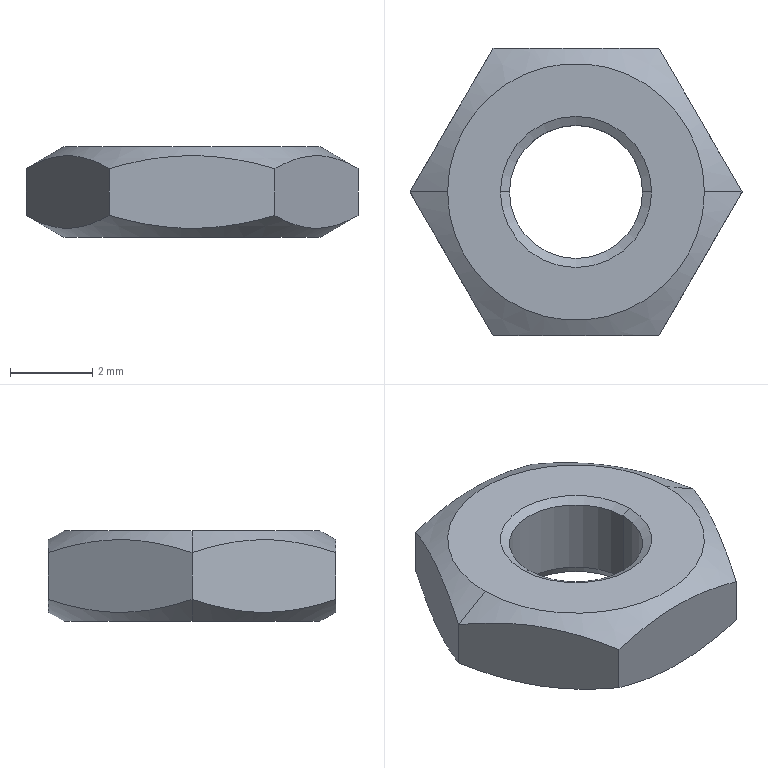Part | SolidWorks | features RevCut 2, Chamfer 1, Extrusion 1, LPattern 1 | 1 solid | 18 faces | box 8.083 x 7 x 2.2 mm | volume 70.72 mm3 | cone 8 | plane 8 | cylinder 2 | commonest cylinder face diameters 3.242 x2
STEP:
#1=CARTESIAN_POINT('',(-1.621,0.,-0.127));
#2=VERTEX_POINT('',#1);
#3=CARTESIAN_POINT('',(1.621,0.,-0.127));
#4=VERTEX_POINT('',#3);
#5=CARTESIAN_POINT('',(0.,0.,-0.127));
#6=DIRECTION('',(0.,0.,1.));
#7=DIRECTION('',(1.,0.,0.));
#8=AXIS2_PLACEMENT_3D('',#5,#6,#7);
#9=CIRCLE('',#8,1.621);
#10=EDGE_CURVE('',#2,#4,#9,.T.);
#11=ORIENTED_EDGE('',*,*,#10,.F.);
#12=CARTESIAN_POINT('',(-1.841,0.,0.));
#13=VERTEX_POINT('',#12);
#14=CARTESIAN_POINT('',(-1.621,0.,-0.127));
#15=DIRECTION('',(-0.866,0.,0.5));
#16=VECTOR('',#15,1000.);
#17=LINE('',#14,#16);
#18=EDGE_CURVE('',#2,#13,#17,.T.);
#19=ORIENTED_EDGE('',*,*,#18,.T.);
#20=CARTESIAN_POINT('',(1.841,0.,0.));
#21=VERTEX_POINT('',#20);
#22=CARTESIAN_POINT('',(0.,0.,0.));
#23=DIRECTION('',(0.,0.,-1.));
#24=DIRECTION('',(1.,0.,0.));
#25=AXIS2_PLACEMENT_3D('',#22,#23,#24);
#26=CIRCLE('',#25,1.841);
#27=EDGE_CURVE('',#21,#13,#26,.T.);
#28=ORIENTED_EDGE('',*,*,#27,.F.);
#29=CARTESIAN_POINT('',(1.621,0.,-0.127));
#30=DIRECTION('',(0.866,0.,0.5));
#31=VECTOR('',#30,1000.);
#32=LINE('',#29,#31);
#33=EDGE_CURVE('',#4,#21,#32,.T.);
#34=ORIENTED_EDGE('',*,*,#33,.F.);
#35=EDGE_LOOP('',(#11,#19,#28,#34));
#36=FACE_OUTER_BOUND('',#35,.T.);
#37=CARTESIAN_POINT('',(0.,0.,-0.127));
#38=DIRECTION('',(0.,0.,1.));
#39=DIRECTION('',(1.,0.,0.));
#40=AXIS2_PLACEMENT_3D('',#37,#38,#39);
#41=CONICAL_SURFACE('',#40,1.621,1.047);
#42=ADVANCED_FACE('',(#36),#41,.F.);
#43=CARTESIAN_POINT('',(1.621,0.,-1.98));
#44=VERTEX_POINT('',#43);
#45=CARTESIAN_POINT('',(-1.621,0.,-1.98));
#46=VERTEX_POINT('',#45);
#47=CARTESIAN_POINT('',(0.,0.,-1.98));
#48=DIRECTION('',(0.,0.,-1.));
#49=DIRECTION('',(1.,0.,0.));
#50=AXIS2_PLACEMENT_3D('',#47,#48,#49);
#51=CIRCLE('',#50,1.621);
#52=EDGE_CURVE('',#44,#46,#51,.T.);
#53=ORIENTED_EDGE('',*,*,#52,.F.);
#54=CARTESIAN_POINT('',(1.748,0.,-2.2));
#55=VERTEX_POINT('',#54);
#56=CARTESIAN_POINT('',(1.748,0.,-2.2));
#57=DIRECTION('',(0.5,0.,-0.866));
#58=VECTOR('',#57,1000.);
#59=LINE('',#56,#58);
#60=EDGE_CURVE('',#44,#55,#59,.T.);
#61=ORIENTED_EDGE('',*,*,#60,.T.);
#62=CARTESIAN_POINT('',(-1.748,0.,-2.2));
#63=VERTEX_POINT('',#62);
#64=CARTESIAN_POINT('',(0.,0.,-2.2));
#65=DIRECTION('',(0.,0.,1.));
#66=DIRECTION('',(1.,0.,0.));
#67=AXIS2_PLACEMENT_3D('',#64,#65,#66);
#68=CIRCLE('',#67,1.748);
#69=EDGE_CURVE('',#63,#55,#68,.T.);
#70=ORIENTED_EDGE('',*,*,#69,.F.);
#71=CARTESIAN_POINT('',(-1.748,0.,-2.2));
#72=DIRECTION('',(-0.5,0.,-0.866));
#73=VECTOR('',#72,1000.);
#74=LINE('',#71,#73);
#75=EDGE_CURVE('',#46,#63,#74,.T.);
#76=ORIENTED_EDGE('',*,*,#75,.F.);
#77=EDGE_LOOP('',(#53,#61,#70,#76));
#78=FACE_OUTER_BOUND('',#77,.T.);
#79=CARTESIAN_POINT('',(0.,0.,-2.2));
#80=DIRECTION('',(0.,0.,-1.));
#81=DIRECTION('',(-1.,0.,0.));
#82=AXIS2_PLACEMENT_3D('',#79,#80,#81);
#83=CONICAL_SURFACE('',#82,1.748,0.5236);
#84=ADVANCED_FACE('',(#78),#83,.F.);
#85=CARTESIAN_POINT('',(-3.125,0.,0.));
#86=VERTEX_POINT('',#85);
#87=CARTESIAN_POINT('',(3.125,0.,0.));
#88=VERTEX_POINT('',#87);
#89=CARTESIAN_POINT('',(0.,0.,0.));
#90=DIRECTION('',(0.,0.,-1.));
#91=DIRECTION('',(-1.,0.,0.));
#92=AXIS2_PLACEMENT_3D('',#89,#90,#91);
#93=CIRCLE('',#92,3.125);
#94=EDGE_CURVE('',#86,#88,#93,.T.);
#95=ORIENTED_EDGE('',*,*,#94,.T.);
#96=CARTESIAN_POINT('',(4.041,0.,-0.5291));
#97=VERTEX_POINT('',#96);
#98=CARTESIAN_POINT('',(3.125,0.,0.));
#99=DIRECTION('',(0.866,0.,-0.5));
#100=VECTOR('',#99,1000.);
#101=LINE('',#98,#100);
#102=EDGE_CURVE('',#88,#97,#101,.T.);
#103=ORIENTED_EDGE('',*,*,#102,.T.);
#104=CARTESIAN_POINT('',(2.021,3.5,-0.5291));
#105=VERTEX_POINT('',#104);
#106=CARTESIAN_POINT('',(4.041,0.,-0.5291));
#107=CARTESIAN_POINT('',(3.712,0.5715,-0.3386));
#108=CARTESIAN_POINT('',(3.377,1.152,-0.2169));
#109=CARTESIAN_POINT('',(2.861,2.044,-0.2163));
#110=CARTESIAN_POINT('',(2.69,2.341,-0.2461));
#111=CARTESIAN_POINT('',(2.352,2.925,-0.3551));
#112=CARTESIAN_POINT('',(2.186,3.214,-0.4337));
#113=CARTESIAN_POINT('',(2.021,3.5,-0.5291));
#114=B_SPLINE_CURVE_WITH_KNOTS('',3,(#106,#107,#108,#109,#110,#111,#112,#113),.UNSPECIFIED.,.F.,.F.,(4,2,2,4),(0.000000238,0.002041,0.003061,0.004082),.UNSPECIFIED.);
#115=EDGE_CURVE('',#97,#105,#114,.T.);
#116=ORIENTED_EDGE('',*,*,#115,.T.);
#117=CARTESIAN_POINT('',(-2.021,3.5,-0.5291));
#118=VERTEX_POINT('',#117);
#119=CARTESIAN_POINT('',(2.021,3.5,-0.5291));
#120=CARTESIAN_POINT('',(1.694,3.5,-0.4348));
#121=CARTESIAN_POINT('',(1.363,3.5,-0.3563));
#122=CARTESIAN_POINT('',(0.6882,3.5,-0.2467));
#123=CARTESIAN_POINT('',(0.342,3.5,-0.2165));
#124=CARTESIAN_POINT('',(-0.3409,3.5,-0.2165));
#125=CARTESIAN_POINT('',(-0.6803,3.5,-0.2458));
#126=CARTESIAN_POINT('',(-1.355,3.5,-0.3546));
#127=CARTESIAN_POINT('',(-1.692,3.5,-0.4342));
#128=CARTESIAN_POINT('',(-2.021,3.5,-0.5291));
#129=B_SPLINE_CURVE_WITH_KNOTS('',3,(#119,#120,#121,#122,#123,#124,#125,#126,#127,#128),.UNSPECIFIED.,.F.,.F.,(4,2,2,2,4),(0.008992,0.01002,0.01104,0.01206,0.01309),.UNSPECIFIED.);
#130=EDGE_CURVE('',#105,#118,#129,.T.);
#131=ORIENTED_EDGE('',*,*,#130,.T.);
#132=CARTESIAN_POINT('',(-4.041,0.,-0.5291));
#133=VERTEX_POINT('',#132);
#134=CARTESIAN_POINT('',(-2.021,3.5,-0.5291));
#135=CARTESIAN_POINT('',(-2.351,2.929,-0.3386));
#136=CARTESIAN_POINT('',(-2.686,2.348,-0.2169));
#137=CARTESIAN_POINT('',(-3.201,1.456,-0.2163));
#138=CARTESIAN_POINT('',(-3.373,1.159,-0.2461));
#139=CARTESIAN_POINT('',(-3.71,0.5746,-0.3551));
#140=CARTESIAN_POINT('',(-3.876,0.2861,-0.4337));
#141=CARTESIAN_POINT('',(-4.041,0.,-0.5291));
#142=B_SPLINE_CURVE_WITH_KNOTS('',3,(#134,#135,#136,#137,#138,#139,#140,#141),.UNSPECIFIED.,.F.,.F.,(4,2,2,4),(0.000000238,0.002041,0.003061,0.004082),.UNSPECIFIED.);
#143=EDGE_CURVE('',#118,#133,#142,.T.);
#144=ORIENTED_EDGE('',*,*,#143,.T.);
#145=CARTESIAN_POINT('',(-3.125,0.,0.));
#146=DIRECTION('',(-0.866,0.,-0.5));
#147=VECTOR('',#146,1000.);
#148=LINE('',#145,#147);
#149=EDGE_CURVE('',#86,#133,#148,.T.);
#150=ORIENTED_EDGE('',*,*,#149,.F.);
#151=EDGE_LOOP('',(#95,#103,#116,#131,#144,#150));
#152=FACE_OUTER_BOUND('',#151,.T.);
#153=CARTESIAN_POINT('',(0.,0.,0.));
#154=DIRECTION('',(0.,0.,-1.));
#155=DIRECTION('',(-1.,0.,0.));
#156=AXIS2_PLACEMENT_3D('',#153,#154,#155);
#157=CONICAL_SURFACE('',#156,3.125,1.047);
#158=ADVANCED_FACE('',(#152),#157,.T.);
#159=CARTESIAN_POINT('',(-3.125,0.,-2.2));
#160=VERTEX_POINT('',#159);
#161=CARTESIAN_POINT('',(3.125,0.,-2.2));
#162=VERTEX_POINT('',#161);
#163=CARTESIAN_POINT('',(0.,0.,-2.2));
#164=DIRECTION('',(0.,0.,-1.));
#165=DIRECTION('',(-1.,0.,0.));
#166=AXIS2_PLACEMENT_3D('',#163,#164,#165);
#167=CIRCLE('',#166,3.125);
#168=EDGE_CURVE('',#160,#162,#167,.T.);
#169=ORIENTED_EDGE('',*,*,#168,.F.);
#170=CARTESIAN_POINT('',(-4.041,0.,-1.671));
#171=VERTEX_POINT('',#170);
#172=CARTESIAN_POINT('',(-4.041,0.,-1.671));
#173=DIRECTION('',(-0.866,0.,0.5));
#174=VECTOR('',#173,1000.);
#175=LINE('',#172,#174);
#176=EDGE_CURVE('',#160,#171,#175,.T.);
#177=ORIENTED_EDGE('',*,*,#176,.T.);
#178=CARTESIAN_POINT('',(-2.021,3.5,-1.671));
#179=VERTEX_POINT('',#178);
#180=CARTESIAN_POINT('',(-4.041,0.,-1.671));
#181=CARTESIAN_POINT('',(-3.712,0.5715,-1.861));
#182=CARTESIAN_POINT('',(-3.377,1.152,-1.983));
#183=CARTESIAN_POINT('',(-2.861,2.044,-1.984));
#184=CARTESIAN_POINT('',(-2.69,2.341,-1.954));
#185=CARTESIAN_POINT('',(-2.352,2.925,-1.845));
#186=CARTESIAN_POINT('',(-2.186,3.214,-1.766));
#187=CARTESIAN_POINT('',(-2.021,3.5,-1.671));
#188=B_SPLINE_CURVE_WITH_KNOTS('',3,(#180,#181,#182,#183,#184,#185,#186,#187),.UNSPECIFIED.,.F.,.F.,(4,2,2,4),(0.000000238,0.002041,0.003061,0.004082),.UNSPECIFIED.);
#189=EDGE_CURVE('',#171,#179,#188,.T.);
#190=ORIENTED_EDGE('',*,*,#189,.T.);
#191=CARTESIAN_POINT('',(2.021,3.5,-1.671));
#192=VERTEX_POINT('',#191);
#193=CARTESIAN_POINT('',(-2.021,3.5,-1.671));
#194=CARTESIAN_POINT('',(-1.692,3.5,-1.766));
#195=CARTESIAN_POINT('',(-1.355,3.5,-1.845));
#196=CARTESIAN_POINT('',(-0.6803,3.5,-1.954));
#197=CARTESIAN_POINT('',(-0.3409,3.5,-1.984));
#198=CARTESIAN_POINT('',(0.342,3.5,-1.983));
#199=CARTESIAN_POINT('',(0.6882,3.5,-1.953));
#200=CARTESIAN_POINT('',(1.363,3.5,-1.844));
#201=CARTESIAN_POINT('',(1.694,3.5,-1.765));
#202=CARTESIAN_POINT('',(2.021,3.5,-1.671));
#203=B_SPLINE_CURVE_WITH_KNOTS('',3,(#193,#194,#195,#196,#197,#198,#199,#200,#201,#202),.UNSPECIFIED.,.F.,.F.,(4,2,2,2,4),(0.003572,0.004594,0.005616,0.006639,0.007661),.UNSPECIFIED.);
#204=EDGE_CURVE('',#179,#192,#203,.T.);
#205=ORIENTED_EDGE('',*,*,#204,.T.);
#206=CARTESIAN_POINT('',(4.041,0.,-1.671));
#207=VERTEX_POINT('',#206);
#208=CARTESIAN_POINT('',(2.021,3.5,-1.671));
#209=CARTESIAN_POINT('',(2.351,2.929,-1.861));
#210=CARTESIAN_POINT('',(2.686,2.348,-1.983));
#211=CARTESIAN_POINT('',(3.201,1.456,-1.984));
#212=CARTESIAN_POINT('',(3.373,1.159,-1.954));
#213=CARTESIAN_POINT('',(3.71,0.5746,-1.845));
#214=CARTESIAN_POINT('',(3.876,0.2861,-1.766));
#215=CARTESIAN_POINT('',(4.041,0.,-1.671));
#216=B_SPLINE_CURVE_WITH_KNOTS('',3,(#208,#209,#210,#211,#212,#213,#214,#215),.UNSPECIFIED.,.F.,.F.,(4,2,2,4),(0.000000238,0.002041,0.003061,0.004082),.UNSPECIFIED.);
#217=EDGE_CURVE('',#192,#207,#216,.T.);
#218=ORIENTED_EDGE('',*,*,#217,.T.);
#219=CARTESIAN_POINT('',(4.041,0.,-1.671));
#220=DIRECTION('',(0.866,0.,0.5));
#221=VECTOR('',#220,1000.);
#222=LINE('',#219,#221);
#223=EDGE_CURVE('',#162,#207,#222,.T.);
#224=ORIENTED_EDGE('',*,*,#223,.F.);
#225=EDGE_LOOP('',(#169,#177,#190,#205,#218,#224));
#226=FACE_OUTER_BOUND('',#225,.T.);
#227=CARTESIAN_POINT('',(0.,0.,-1.671));
#228=DIRECTION('',(0.,0.,1.));
#229=DIRECTION('',(1.,0.,0.));
#230=AXIS2_PLACEMENT_3D('',#227,#228,#229);
#231=CONICAL_SURFACE('',#230,4.041,1.047);
#232=ADVANCED_FACE('',(#226),#231,.T.);
#233=ORIENTED_EDGE('',*,*,#52,.T.);
#234=CARTESIAN_POINT('',(-1.621,0.,-2.2));
#235=DIRECTION('',(0.,0.,1.));
#236=VECTOR('',#235,1000.);
#237=LINE('',#234,#236);
#238=EDGE_CURVE('',#46,#2,#237,.T.);
#239=ORIENTED_EDGE('',*,*,#238,.T.);
#240=ORIENTED_EDGE('',*,*,#10,.T.);
#241=CARTESIAN_POINT('',(1.621,0.,-2.2));
#242=DIRECTION('',(0.,0.,1.));
#243=VECTOR('',#242,1000.);
#244=LINE('',#241,#243);
#245=EDGE_CURVE('',#44,#4,#244,.T.);
#246=ORIENTED_EDGE('',*,*,#245,.F.);
#247=EDGE_LOOP('',(#233,#239,#240,#246));
#248=FACE_OUTER_BOUND('',#247,.T.);
#249=CARTESIAN_POINT('',(0.,0.,-2.2));
#250=DIRECTION('',(0.,0.,1.));
#251=DIRECTION('',(1.,0.,0.));
#252=AXIS2_PLACEMENT_3D('',#249,#250,#251);
#253=CYLINDRICAL_SURFACE('',#252,1.621);
#254=ADVANCED_FACE('',(#248),#253,.F.);
#255=CARTESIAN_POINT('',(-2.021,-3.5,-0.5291));
#256=VERTEX_POINT('',#255);
#257=CARTESIAN_POINT('',(2.021,-3.5,-0.5291));
#258=VERTEX_POINT('',#257);
#259=CARTESIAN_POINT('',(-2.021,-3.5,-0.5291));
#260=CARTESIAN_POINT('',(-1.692,-3.5,-0.4342));
#261=CARTESIAN_POINT('',(-1.355,-3.5,-0.3546));
#262=CARTESIAN_POINT('',(-0.6803,-3.5,-0.2458));
#263=CARTESIAN_POINT('',(-0.3409,-3.5,-0.2165));
#264=CARTESIAN_POINT('',(0.342,-3.5,-0.2165));
#265=CARTESIAN_POINT('',(0.6882,-3.5,-0.2467));
#266=CARTESIAN_POINT('',(1.363,-3.5,-0.3563));
#267=CARTESIAN_POINT('',(1.694,-3.5,-0.4348));
#268=CARTESIAN_POINT('',(2.021,-3.5,-0.5291));
#269=B_SPLINE_CURVE_WITH_KNOTS('',3,(#259,#260,#261,#262,#263,#264,#265,#266,#267,#268),.UNSPECIFIED.,.F.,.F.,(4,2,2,2,4),(0.003572,0.004594,0.005616,0.006639,0.007661),.UNSPECIFIED.);
#270=EDGE_CURVE('',#256,#258,#269,.T.);
#271=ORIENTED_EDGE('',*,*,#270,.F.);
#272=CARTESIAN_POINT('',(-2.021,-3.5,-1.671));
#273=VERTEX_POINT('',#272);
#274=CARTESIAN_POINT('',(-2.021,-3.5,-2.2));
#275=DIRECTION('',(0.,0.,1.));
#276=VECTOR('',#275,1000.);
#277=LINE('',#274,#276);
#278=EDGE_CURVE('',#273,#256,#277,.T.);
#279=ORIENTED_EDGE('',*,*,#278,.F.);
#280=CARTESIAN_POINT('',(2.021,-3.5,-1.671));
#281=VERTEX_POINT('',#280);
#282=CARTESIAN_POINT('',(2.021,-3.5,-1.671));
#283=CARTESIAN_POINT('',(1.694,-3.5,-1.765));
#284=CARTESIAN_POINT('',(1.363,-3.5,-1.844));
#285=CARTESIAN_POINT('',(0.6882,-3.5,-1.953));
#286=CARTESIAN_POINT('',(0.342,-3.5,-1.983));
#287=CARTESIAN_POINT('',(-0.3409,-3.5,-1.984));
#288=CARTESIAN_POINT('',(-0.6803,-3.5,-1.954));
#289=CARTESIAN_POINT('',(-1.355,-3.5,-1.845));
#290=CARTESIAN_POINT('',(-1.692,-3.5,-1.766));
#291=CARTESIAN_POINT('',(-2.021,-3.5,-1.671));
#292=B_SPLINE_CURVE_WITH_KNOTS('',3,(#282,#283,#284,#285,#286,#287,#288,#289,#290,#291),.UNSPECIFIED.,.F.,.F.,(4,2,2,2,4),(0.008992,0.01002,0.01104,0.01206,0.01309),.UNSPECIFIED.);
#293=EDGE_CURVE('',#281,#273,#292,.T.);
#294=ORIENTED_EDGE('',*,*,#293,.F.);
#295=CARTESIAN_POINT('',(2.021,-3.5,-2.2));
#296=DIRECTION('',(0.,0.,1.));
#297=VECTOR('',#296,1000.);
#298=LINE('',#295,#297);
#299=EDGE_CURVE('',#281,#258,#298,.T.);
#300=ORIENTED_EDGE('',*,*,#299,.T.);
#301=EDGE_LOOP('',(#271,#279,#294,#300));
#302=FACE_OUTER_BOUND('',#301,.T.);
#303=CARTESIAN_POINT('',(-2.021,-3.5,-2.2));
#304=DIRECTION('',(0.,-1.,0.));
#305=DIRECTION('',(1.,0.,0.));
#306=AXIS2_PLACEMENT_3D('',#303,#304,#305);
#307=PLANE('',#306);
#308=ADVANCED_FACE('',(#302),#307,.T.);
#309=CARTESIAN_POINT('',(-4.041,0.,-0.5291));
#310=CARTESIAN_POINT('',(-3.712,-0.5715,-0.3386));
#311=CARTESIAN_POINT('',(-3.377,-1.152,-0.2169));
#312=CARTESIAN_POINT('',(-2.861,-2.044,-0.2163));
#313=CARTESIAN_POINT('',(-2.69,-2.341,-0.2461));
#314=CARTESIAN_POINT('',(-2.352,-2.925,-0.3551));
#315=CARTESIAN_POINT('',(-2.186,-3.214,-0.4337));
#316=CARTESIAN_POINT('',(-2.021,-3.5,-0.5291));
#317=B_SPLINE_CURVE_WITH_KNOTS('',3,(#309,#310,#311,#312,#313,#314,#315,#316),.UNSPECIFIED.,.F.,.F.,(4,2,2,4),(0.000000238,0.002041,0.003061,0.004082),.UNSPECIFIED.);
#318=EDGE_CURVE('',#133,#256,#317,.T.);
#319=ORIENTED_EDGE('',*,*,#318,.F.);
#320=CARTESIAN_POINT('',(-4.041,0.,-2.2));
#321=DIRECTION('',(0.,0.,1.));
#322=VECTOR('',#321,1000.);
#323=LINE('',#320,#322);
#324=EDGE_CURVE('',#171,#133,#323,.T.);
#325=ORIENTED_EDGE('',*,*,#324,.F.);
#326=CARTESIAN_POINT('',(-2.021,-3.5,-1.671));
#327=CARTESIAN_POINT('',(-2.351,-2.929,-1.861));
#328=CARTESIAN_POINT('',(-2.686,-2.348,-1.983));
#329=CARTESIAN_POINT('',(-3.201,-1.456,-1.984));
#330=CARTESIAN_POINT('',(-3.373,-1.159,-1.954));
#331=CARTESIAN_POINT('',(-3.71,-0.5746,-1.845));
#332=CARTESIAN_POINT('',(-3.876,-0.2861,-1.766));
#333=CARTESIAN_POINT('',(-4.041,0.,-1.671));
#334=B_SPLINE_CURVE_WITH_KNOTS('',3,(#326,#327,#328,#329,#330,#331,#332,#333),.UNSPECIFIED.,.F.,.F.,(4,2,2,4),(0.000000238,0.002041,0.003061,0.004082),.UNSPECIFIED.);
#335=EDGE_CURVE('',#273,#171,#334,.T.);
#336=ORIENTED_EDGE('',*,*,#335,.F.);
#337=ORIENTED_EDGE('',*,*,#278,.T.);
#338=EDGE_LOOP('',(#319,#325,#336,#337));
#339=FACE_OUTER_BOUND('',#338,.T.);
#340=CARTESIAN_POINT('',(-4.041,0.,-2.2));
#341=DIRECTION('',(-0.866,-0.5,0.));
#342=DIRECTION('',(0.5,-0.866,0.));
#343=AXIS2_PLACEMENT_3D('',#340,#341,#342);
#344=PLANE('',#343);
#345=ADVANCED_FACE('',(#339),#344,.T.);
#346=ORIENTED_EDGE('',*,*,#143,.F.);
#347=CARTESIAN_POINT('',(-2.021,3.5,-2.2));
#348=DIRECTION('',(0.,0.,1.));
#349=VECTOR('',#348,1000.);
#350=LINE('',#347,#349);
#351=EDGE_CURVE('',#179,#118,#350,.T.);
#352=ORIENTED_EDGE('',*,*,#351,.F.);
#353=ORIENTED_EDGE('',*,*,#189,.F.);
#354=ORIENTED_EDGE('',*,*,#324,.T.);
#355=EDGE_LOOP('',(#346,#352,#353,#354));
#356=FACE_OUTER_BOUND('',#355,.T.);
#357=CARTESIAN_POINT('',(-2.021,3.5,-2.2));
#358=DIRECTION('',(-0.866,0.5,0.));
#359=DIRECTION('',(-0.5,-0.866,0.));
#360=AXIS2_PLACEMENT_3D('',#357,#358,#359);
#361=PLANE('',#360);
#362=ADVANCED_FACE('',(#356),#361,.T.);
#363=ORIENTED_EDGE('',*,*,#130,.F.);
#364=CARTESIAN_POINT('',(2.021,3.5,-2.2));
#365=DIRECTION('',(0.,0.,1.));
#366=VECTOR('',#365,1000.);
#367=LINE('',#364,#366);
#368=EDGE_CURVE('',#192,#105,#367,.T.);
#369=ORIENTED_EDGE('',*,*,#368,.F.);
#370=ORIENTED_EDGE('',*,*,#204,.F.);
#371=ORIENTED_EDGE('',*,*,#351,.T.);
#372=EDGE_LOOP('',(#363,#369,#370,#371));
#373=FACE_OUTER_BOUND('',#372,.T.);
#374=CARTESIAN_POINT('',(2.021,3.5,-2.2));
#375=DIRECTION('',(0.,1.,0.));
#376=DIRECTION('',(0.,0.,1.));
#377=AXIS2_PLACEMENT_3D('',#374,#375,#376);
#378=PLANE('',#377);
#379=ADVANCED_FACE('',(#373),#378,.T.);
#380=ORIENTED_EDGE('',*,*,#115,.F.);
#381=CARTESIAN_POINT('',(4.041,0.,-2.2));
#382=DIRECTION('',(0.,0.,1.));
#383=VECTOR('',#382,1000.);
#384=LINE('',#381,#383);
#385=EDGE_CURVE('',#207,#97,#384,.T.);
#386=ORIENTED_EDGE('',*,*,#385,.F.);
#387=ORIENTED_EDGE('',*,*,#217,.F.);
#388=ORIENTED_EDGE('',*,*,#368,.T.);
#389=EDGE_LOOP('',(#380,#386,#387,#388));
#390=FACE_OUTER_BOUND('',#389,.T.);
#391=CARTESIAN_POINT('',(4.041,0.,-2.2));
#392=DIRECTION('',(0.866,0.5,0.));
#393=DIRECTION('',(-0.5,0.866,0.));
#394=AXIS2_PLACEMENT_3D('',#391,#392,#393);
#395=PLANE('',#394);
#396=ADVANCED_FACE('',(#390),#395,.T.);
#397=CARTESIAN_POINT('',(2.021,-3.5,-0.5291));
#398=CARTESIAN_POINT('',(2.351,-2.929,-0.3386));
#399=CARTESIAN_POINT('',(2.686,-2.348,-0.2169));
#400=CARTESIAN_POINT('',(3.201,-1.456,-0.2163));
#401=CARTESIAN_POINT('',(3.373,-1.159,-0.2461));
#402=CARTESIAN_POINT('',(3.71,-0.5746,-0.3551));
#403=CARTESIAN_POINT('',(3.876,-0.2861,-0.4337));
#404=CARTESIAN_POINT('',(4.041,0.,-0.5291));
#405=B_SPLINE_CURVE_WITH_KNOTS('',3,(#397,#398,#399,#400,#401,#402,#403,#404),.UNSPECIFIED.,.F.,.F.,(4,2,2,4),(0.000000238,0.002041,0.003061,0.004082),.UNSPECIFIED.);
#406=EDGE_CURVE('',#258,#97,#405,.T.);
#407=ORIENTED_EDGE('',*,*,#406,.F.);
#408=ORIENTED_EDGE('',*,*,#299,.F.);
#409=CARTESIAN_POINT('',(4.041,0.,-1.671));
#410=CARTESIAN_POINT('',(3.712,-0.5715,-1.861));
#411=CARTESIAN_POINT('',(3.377,-1.152,-1.983));
#412=CARTESIAN_POINT('',(2.861,-2.044,-1.984));
#413=CARTESIAN_POINT('',(2.69,-2.341,-1.954));
#414=CARTESIAN_POINT('',(2.352,-2.925,-1.845));
#415=CARTESIAN_POINT('',(2.186,-3.214,-1.766));
#416=CARTESIAN_POINT('',(2.021,-3.5,-1.671));
#417=B_SPLINE_CURVE_WITH_KNOTS('',3,(#409,#410,#411,#412,#413,#414,#415,#416),.UNSPECIFIED.,.F.,.F.,(4,2,2,4),(0.000000238,0.002041,0.003061,0.004082),.UNSPECIFIED.);
#418=EDGE_CURVE('',#207,#281,#417,.T.);
#419=ORIENTED_EDGE('',*,*,#418,.F.);
#420=ORIENTED_EDGE('',*,*,#385,.T.);
#421=EDGE_LOOP('',(#407,#408,#419,#420));
#422=FACE_OUTER_BOUND('',#421,.T.);
#423=CARTESIAN_POINT('',(2.021,-3.5,-2.2));
#424=DIRECTION('',(0.866,-0.5,0.));
#425=DIRECTION('',(0.5,0.866,0.));
#426=AXIS2_PLACEMENT_3D('',#423,#424,#425);
#427=PLANE('',#426);
#428=ADVANCED_FACE('',(#422),#427,.T.);
#429=ORIENTED_EDGE('',*,*,#69,.T.);
#430=CARTESIAN_POINT('',(0.,0.,-2.2));
#431=DIRECTION('',(0.,0.,1.));
#432=DIRECTION('',(1.,0.,0.));
#433=AXIS2_PLACEMENT_3D('',#430,#431,#432);
#434=CIRCLE('',#433,1.748);
#435=EDGE_CURVE('',#55,#63,#434,.T.);
#436=ORIENTED_EDGE('',*,*,#435,.T.);
#437=EDGE_LOOP('',(#429,#436));
#438=FACE_BOUND('',#437,.T.);
#439=CARTESIAN_POINT('',(0.,0.,-2.2));
#440=DIRECTION('',(0.,0.,-1.));
#441=DIRECTION('',(-1.,0.,0.));
#442=AXIS2_PLACEMENT_3D('',#439,#440,#441);
#443=CIRCLE('',#442,3.125);
#444=EDGE_CURVE('',#162,#160,#443,.T.);
#445=ORIENTED_EDGE('',*,*,#444,.T.);
#446=ORIENTED_EDGE('',*,*,#168,.T.);
#447=EDGE_LOOP('',(#445,#446));
#448=FACE_OUTER_BOUND('',#447,.T.);
#449=CARTESIAN_POINT('',(2.021,-3.5,-2.2));
#450=DIRECTION('',(0.,0.,1.));
#451=DIRECTION('',(1.,0.,0.));
#452=AXIS2_PLACEMENT_3D('',#449,#450,#451);
#453=PLANE('',#452);
#454=ADVANCED_FACE('',(#438,#448),#453,.F.);
#455=ORIENTED_EDGE('',*,*,#27,.T.);
#456=CARTESIAN_POINT('',(0.,0.,0.));
#457=DIRECTION('',(0.,0.,-1.));
#458=DIRECTION('',(1.,0.,0.));
#459=AXIS2_PLACEMENT_3D('',#456,#457,#458);
#460=CIRCLE('',#459,1.841);
#461=EDGE_CURVE('',#13,#21,#460,.T.);
#462=ORIENTED_EDGE('',*,*,#461,.T.);
#463=EDGE_LOOP('',(#455,#462));
#464=FACE_BOUND('',#463,.T.);
#465=ORIENTED_EDGE('',*,*,#94,.F.);
#466=CARTESIAN_POINT('',(0.,0.,0.));
#467=DIRECTION('',(0.,0.,-1.));
#468=DIRECTION('',(-1.,0.,0.));
#469=AXIS2_PLACEMENT_3D('',#466,#467,#468);
#470=CIRCLE('',#469,3.125);
#471=EDGE_CURVE('',#88,#86,#470,.T.);
#472=ORIENTED_EDGE('',*,*,#471,.F.);
#473=EDGE_LOOP('',(#465,#472));
#474=FACE_OUTER_BOUND('',#473,.T.);
#475=CARTESIAN_POINT('',(2.021,-3.5,0.));
#476=DIRECTION('',(0.,0.,1.));
#477=DIRECTION('',(1.,0.,0.));
#478=AXIS2_PLACEMENT_3D('',#475,#476,#477);
#479=PLANE('',#478);
#480=ADVANCED_FACE('',(#464,#474),#479,.T.);
#481=ORIENTED_EDGE('',*,*,#238,.F.);
#482=CARTESIAN_POINT('',(0.,0.,-1.98));
#483=DIRECTION('',(0.,0.,-1.));
#484=DIRECTION('',(1.,0.,0.));
#485=AXIS2_PLACEMENT_3D('',#482,#483,#484);
#486=CIRCLE('',#485,1.621);
#487=EDGE_CURVE('',#46,#44,#486,.T.);
#488=ORIENTED_EDGE('',*,*,#487,.T.);
#489=ORIENTED_EDGE('',*,*,#245,.T.);
#490=CARTESIAN_POINT('',(0.,0.,-0.127));
#491=DIRECTION('',(0.,0.,1.));
#492=DIRECTION('',(1.,0.,0.));
#493=AXIS2_PLACEMENT_3D('',#490,#491,#492);
#494=CIRCLE('',#493,1.621);
#495=EDGE_CURVE('',#4,#2,#494,.T.);
#496=ORIENTED_EDGE('',*,*,#495,.T.);
#497=EDGE_LOOP('',(#481,#488,#489,#496));
#498=FACE_OUTER_BOUND('',#497,.T.);
#499=CARTESIAN_POINT('',(0.,0.,-2.2));
#500=DIRECTION('',(0.,0.,1.));
#501=DIRECTION('',(1.,0.,0.));
#502=AXIS2_PLACEMENT_3D('',#499,#500,#501);
#503=CYLINDRICAL_SURFACE('',#502,1.621);
#504=ADVANCED_FACE('',(#498),#503,.F.);
#505=ORIENTED_EDGE('',*,*,#176,.F.);
#506=ORIENTED_EDGE('',*,*,#444,.F.);
#507=ORIENTED_EDGE('',*,*,#223,.T.);
#508=ORIENTED_EDGE('',*,*,#418,.T.);
#509=ORIENTED_EDGE('',*,*,#293,.T.);
#510=ORIENTED_EDGE('',*,*,#335,.T.);
#511=EDGE_LOOP('',(#505,#506,#507,#508,#509,#510));
#512=FACE_OUTER_BOUND('',#511,.T.);
#513=CARTESIAN_POINT('',(0.,0.,-1.671));
#514=DIRECTION('',(0.,0.,1.));
#515=DIRECTION('',(1.,0.,0.));
#516=AXIS2_PLACEMENT_3D('',#513,#514,#515);
#517=CONICAL_SURFACE('',#516,4.041,1.047);
#518=ADVANCED_FACE('',(#512),#517,.T.);
#519=ORIENTED_EDGE('',*,*,#102,.F.);
#520=ORIENTED_EDGE('',*,*,#471,.T.);
#521=ORIENTED_EDGE('',*,*,#149,.T.);
#522=ORIENTED_EDGE('',*,*,#318,.T.);
#523=ORIENTED_EDGE('',*,*,#270,.T.);
#524=ORIENTED_EDGE('',*,*,#406,.T.);
#525=EDGE_LOOP('',(#519,#520,#521,#522,#523,#524));
#526=FACE_OUTER_BOUND('',#525,.T.);
#527=CARTESIAN_POINT('',(0.,0.,0.));
#528=DIRECTION('',(0.,0.,-1.));
#529=DIRECTION('',(-1.,0.,0.));
#530=AXIS2_PLACEMENT_3D('',#527,#528,#529);
#531=CONICAL_SURFACE('',#530,3.125,1.047);
#532=ADVANCED_FACE('',(#526),#531,.T.);
#533=ORIENTED_EDGE('',*,*,#60,.F.);
#534=ORIENTED_EDGE('',*,*,#487,.F.);
#535=ORIENTED_EDGE('',*,*,#75,.T.);
#536=ORIENTED_EDGE('',*,*,#435,.F.);
#537=EDGE_LOOP('',(#533,#534,#535,#536));
#538=FACE_OUTER_BOUND('',#537,.T.);
#539=CARTESIAN_POINT('',(0.,0.,-2.2));
#540=DIRECTION('',(0.,0.,-1.));
#541=DIRECTION('',(-1.,0.,0.));
#542=AXIS2_PLACEMENT_3D('',#539,#540,#541);
#543=CONICAL_SURFACE('',#542,1.748,0.5236);
#544=ADVANCED_FACE('',(#538),#543,.F.);
#545=ORIENTED_EDGE('',*,*,#18,.F.);
#546=ORIENTED_EDGE('',*,*,#495,.F.);
#547=ORIENTED_EDGE('',*,*,#33,.T.);
#548=ORIENTED_EDGE('',*,*,#461,.F.);
#549=EDGE_LOOP('',(#545,#546,#547,#548));
#550=FACE_OUTER_BOUND('',#549,.T.);
#551=CARTESIAN_POINT('',(0.,0.,-0.127));
#552=DIRECTION('',(0.,0.,1.));
#553=DIRECTION('',(1.,0.,0.));
#554=AXIS2_PLACEMENT_3D('',#551,#552,#553);
#555=CONICAL_SURFACE('',#554,1.621,1.047);
#556=ADVANCED_FACE('',(#550),#555,.F.);
#557=CLOSED_SHELL('',(#42,#84,#158,#232,#254,#308,#345,#362,#379,#396,#428,#454,#480,#504,#518,#532,#544,#556));
#558=MANIFOLD_SOLID_BREP('',#557);
#559=CARTESIAN_POINT('',(0.,0.,0.));
#560=DIRECTION('',(0.,0.,1.));
#561=DIRECTION('',(1.,0.,0.));
#562=AXIS2_PLACEMENT_3D('',#559,#560,#561);
#563=(LENGTH_UNIT()NAMED_UNIT(*)SI_UNIT(.MILLI.,.METRE.));
#564=UNCERTAINTY_MEASURE_WITH_UNIT(LENGTH_MEASURE(0.00001),#563,'','');
#565=(NAMED_UNIT(*)PLANE_ANGLE_UNIT()SI_UNIT($,.RADIAN.));
#566=(NAMED_UNIT(*)SI_UNIT($,.STERADIAN.)SOLID_ANGLE_UNIT());
#567=(GEOMETRIC_REPRESENTATION_CONTEXT(3)GLOBAL_UNCERTAINTY_ASSIGNED_CONTEXT((#564))GLOBAL_UNIT_ASSIGNED_CONTEXT((#563,#565,#566))REPRESENTATION_CONTEXT('',''));
#568=ADVANCED_BREP_SHAPE_REPRESENTATION('',(#558,#562),#567);